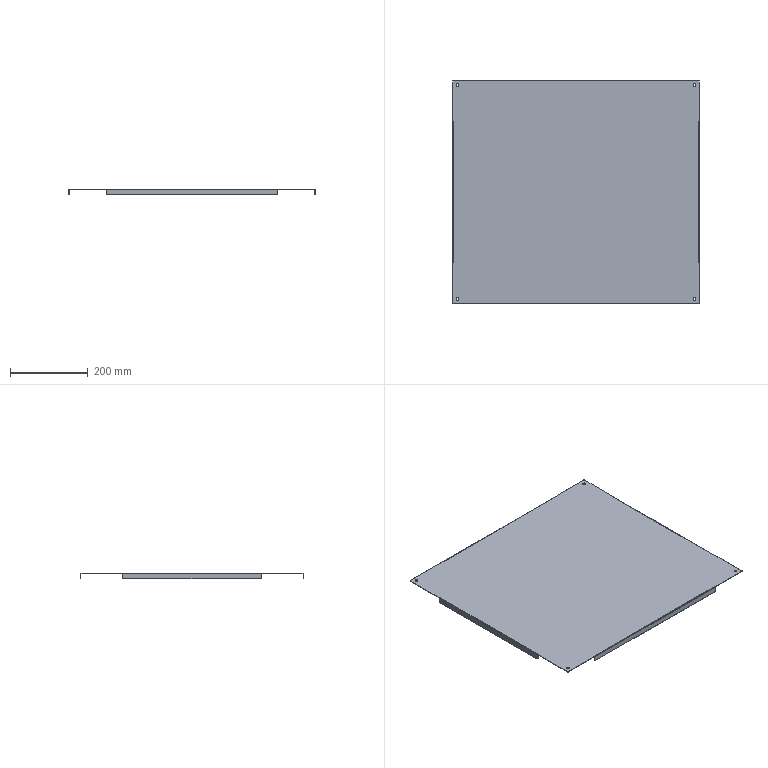Part | SolidWorks | features BaseBody 1 | 1 solid | 90 faces | box 635 x 575 x 15 mm | volume 463497 mm3 | plane 62 | cylinder 28 | commonest cylinder face diameters 7 x8 10 x8 1 x4 3.4 x4 4 x4